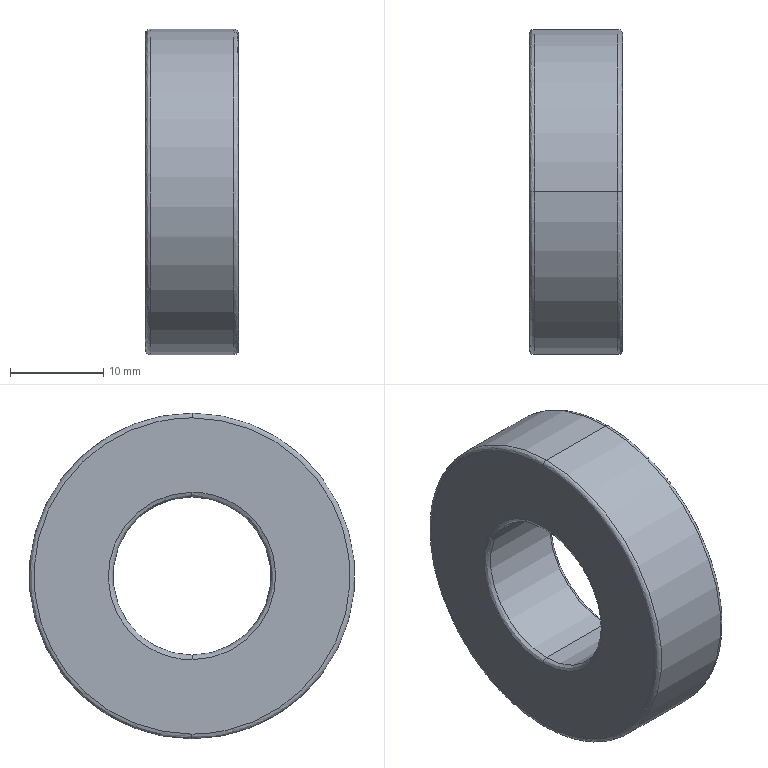Part | STEP file | Bearing B6003ZZ | 1 solid | 14 faces | box 10 x 35 x 35 mm | volume 7334 mm3 | spline 8 | cylinder 4 | plane 2 | commonest cylinder face diameters 17 x2 35 x2